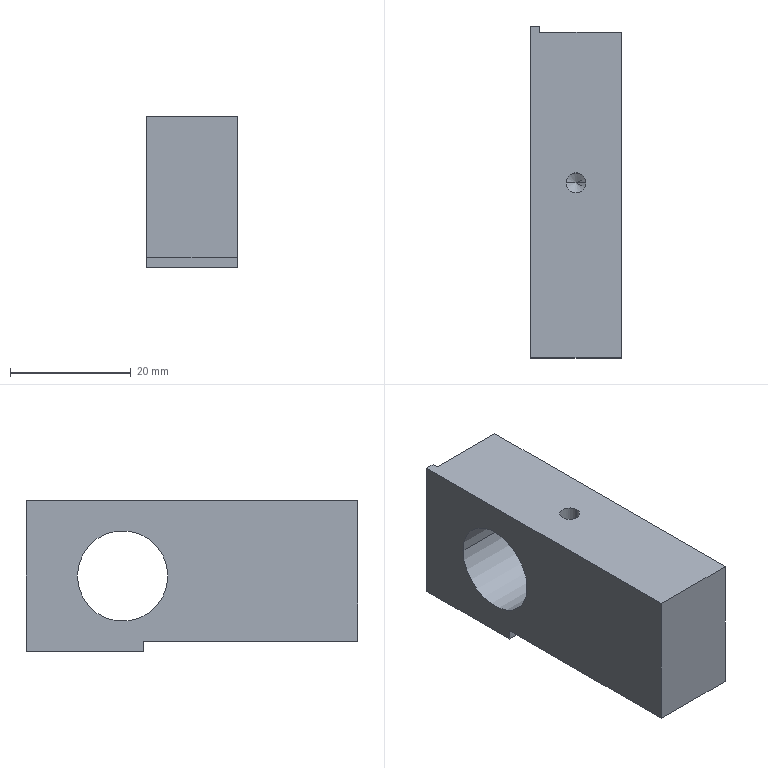Part | STEP file | 11-FG-B07911 | 1 solid | 40 faces | box 15 x 55 x 25 mm | volume 16309 mm3 | cylinder 16 | cone 14 | plane 10 | commonest cylinder face diameters 2.5 x8 3.3 x6 15 x2
STEP:
#1=CARTESIAN_POINT('',(4.7,0.35,9.2));
#2=VERTEX_POINT('',#1);
#3=CARTESIAN_POINT('',(4.7,2.85,9.2));
#4=VERTEX_POINT('',#3);
#5=CARTESIAN_POINT('',(4.7,1.6,9.2));
#6=DIRECTION('',(0.,0.,-1.));
#7=DIRECTION('',(0.,1.,0.));
#8=AXIS2_PLACEMENT_3D('',#5,#6,#7);
#9=CIRCLE('',#8,1.25);
#10=EDGE_CURVE('',#2,#4,#9,.T.);
#11=ORIENTED_EDGE('',*,*,#10,.F.);
#12=CARTESIAN_POINT('',(4.7,0.35,1.7));
#13=VERTEX_POINT('',#12);
#14=CARTESIAN_POINT('',(4.7,0.35,1.7));
#15=DIRECTION('',(0.,0.,-1.));
#16=VECTOR('',#15,1000.);
#17=LINE('',#14,#16);
#18=EDGE_CURVE('',#2,#13,#17,.T.);
#19=ORIENTED_EDGE('',*,*,#18,.T.);
#20=CARTESIAN_POINT('',(4.7,2.85,1.7));
#21=VERTEX_POINT('',#20);
#22=CARTESIAN_POINT('',(4.7,1.6,1.7));
#23=DIRECTION('',(0.,0.,-1.));
#24=DIRECTION('',(0.,1.,0.));
#25=AXIS2_PLACEMENT_3D('',#22,#23,#24);
#26=CIRCLE('',#25,1.25);
#27=EDGE_CURVE('',#13,#21,#26,.T.);
#28=ORIENTED_EDGE('',*,*,#27,.T.);
#29=CARTESIAN_POINT('',(4.7,2.85,1.7));
#30=DIRECTION('',(0.,0.,-1.));
#31=VECTOR('',#30,1000.);
#32=LINE('',#29,#31);
#33=EDGE_CURVE('',#4,#21,#32,.T.);
#34=ORIENTED_EDGE('',*,*,#33,.F.);
#35=EDGE_LOOP('',(#11,#19,#28,#34));
#36=FACE_OUTER_BOUND('',#35,.T.);
#37=CARTESIAN_POINT('',(4.7,1.6,1.7));
#38=DIRECTION('',(0.,0.,-1.));
#39=DIRECTION('',(0.,1.,0.));
#40=AXIS2_PLACEMENT_3D('',#37,#38,#39);
#41=CYLINDRICAL_SURFACE('',#40,1.25);
#42=ADVANCED_FACE('',(#36),#41,.F.);
#43=CARTESIAN_POINT('',(4.7,1.6,9.951));
#44=VERTEX_POINT('',#43);
#45=CARTESIAN_POINT('',(4.7,2.85,9.2));
#46=DIRECTION('',(0.,0.8572,-0.515));
#47=VECTOR('',#46,1000.);
#48=LINE('',#45,#47);
#49=EDGE_CURVE('',#44,#4,#48,.T.);
#50=ORIENTED_EDGE('',*,*,#49,.F.);
#51=CARTESIAN_POINT('',(4.7,0.35,9.2));
#52=DIRECTION('',(0.,-0.8572,-0.515));
#53=VECTOR('',#52,1000.);
#54=LINE('',#51,#53);
#55=EDGE_CURVE('',#44,#2,#54,.T.);
#56=ORIENTED_EDGE('',*,*,#55,.T.);
#57=ORIENTED_EDGE('',*,*,#10,.T.);
#58=EDGE_LOOP('',(#50,#56,#57));
#59=FACE_OUTER_BOUND('',#58,.T.);
#60=CARTESIAN_POINT('',(4.7,1.6,9.2));
#61=DIRECTION('',(0.,0.,-1.));
#62=DIRECTION('',(0.,1.,0.));
#63=AXIS2_PLACEMENT_3D('',#60,#61,#62);
#64=CONICAL_SURFACE('',#63,1.25,1.03);
#65=ADVANCED_FACE('',(#59),#64,.F.);
#66=CARTESIAN_POINT('',(4.7,-19.65,9.2));
#67=VERTEX_POINT('',#66);
#68=CARTESIAN_POINT('',(4.7,-17.15,9.2));
#69=VERTEX_POINT('',#68);
#70=CARTESIAN_POINT('',(4.7,-18.4,9.2));
#71=DIRECTION('',(0.,0.,-1.));
#72=DIRECTION('',(0.,1.,0.));
#73=AXIS2_PLACEMENT_3D('',#70,#71,#72);
#74=CIRCLE('',#73,1.25);
#75=EDGE_CURVE('',#67,#69,#74,.T.);
#76=ORIENTED_EDGE('',*,*,#75,.F.);
#77=CARTESIAN_POINT('',(4.7,-19.65,1.7));
#78=VERTEX_POINT('',#77);
#79=CARTESIAN_POINT('',(4.7,-19.65,1.7));
#80=DIRECTION('',(0.,0.,-1.));
#81=VECTOR('',#80,1000.);
#82=LINE('',#79,#81);
#83=EDGE_CURVE('',#67,#78,#82,.T.);
#84=ORIENTED_EDGE('',*,*,#83,.T.);
#85=CARTESIAN_POINT('',(4.7,-17.15,1.7));
#86=VERTEX_POINT('',#85);
#87=CARTESIAN_POINT('',(4.7,-18.4,1.7));
#88=DIRECTION('',(0.,0.,-1.));
#89=DIRECTION('',(0.,1.,0.));
#90=AXIS2_PLACEMENT_3D('',#87,#88,#89);
#91=CIRCLE('',#90,1.25);
#92=EDGE_CURVE('',#78,#86,#91,.T.);
#93=ORIENTED_EDGE('',*,*,#92,.T.);
#94=CARTESIAN_POINT('',(4.7,-17.15,1.7));
#95=DIRECTION('',(0.,0.,-1.));
#96=VECTOR('',#95,1000.);
#97=LINE('',#94,#96);
#98=EDGE_CURVE('',#69,#86,#97,.T.);
#99=ORIENTED_EDGE('',*,*,#98,.F.);
#100=EDGE_LOOP('',(#76,#84,#93,#99));
#101=FACE_OUTER_BOUND('',#100,.T.);
#102=CARTESIAN_POINT('',(4.7,-18.4,1.7));
#103=DIRECTION('',(0.,0.,-1.));
#104=DIRECTION('',(0.,1.,0.));
#105=AXIS2_PLACEMENT_3D('',#102,#103,#104);
#106=CYLINDRICAL_SURFACE('',#105,1.25);
#107=ADVANCED_FACE('',(#101),#106,.F.);
#108=CARTESIAN_POINT('',(4.7,-18.4,9.951));
#109=VERTEX_POINT('',#108);
#110=CARTESIAN_POINT('',(4.7,-17.15,9.2));
#111=DIRECTION('',(0.,0.8572,-0.515));
#112=VECTOR('',#111,1000.);
#113=LINE('',#110,#112);
#114=EDGE_CURVE('',#109,#69,#113,.T.);
#115=ORIENTED_EDGE('',*,*,#114,.F.);
#116=CARTESIAN_POINT('',(4.7,-19.65,9.2));
#117=DIRECTION('',(0.,-0.8572,-0.515));
#118=VECTOR('',#117,1000.);
#119=LINE('',#116,#118);
#120=EDGE_CURVE('',#109,#67,#119,.T.);
#121=ORIENTED_EDGE('',*,*,#120,.T.);
#122=ORIENTED_EDGE('',*,*,#75,.T.);
#123=EDGE_LOOP('',(#115,#121,#122));
#124=FACE_OUTER_BOUND('',#123,.T.);
#125=CARTESIAN_POINT('',(4.7,-18.4,9.2));
#126=DIRECTION('',(0.,0.,-1.));
#127=DIRECTION('',(0.,1.,0.));
#128=AXIS2_PLACEMENT_3D('',#125,#126,#127);
#129=CONICAL_SURFACE('',#128,1.25,1.03);
#130=ADVANCED_FACE('',(#124),#129,.F.);
#131=CARTESIAN_POINT('',(5.85,5.,14.9));
#132=VERTEX_POINT('',#131);
#133=CARTESIAN_POINT('',(9.15,5.,14.9));
#134=VERTEX_POINT('',#133);
#135=CARTESIAN_POINT('',(7.5,5.,14.9));
#136=DIRECTION('',(0.,0.,1.));
#137=DIRECTION('',(1.,0.,0.));
#138=AXIS2_PLACEMENT_3D('',#135,#136,#137);
#139=CIRCLE('',#138,1.65);
#140=EDGE_CURVE('',#132,#134,#139,.T.);
#141=ORIENTED_EDGE('',*,*,#140,.F.);
#142=CARTESIAN_POINT('',(5.85,5.,25.));
#143=VERTEX_POINT('',#142);
#144=CARTESIAN_POINT('',(5.85,5.,25.));
#145=DIRECTION('',(0.,0.,1.));
#146=VECTOR('',#145,1000.);
#147=LINE('',#144,#146);
#148=EDGE_CURVE('',#132,#143,#147,.T.);
#149=ORIENTED_EDGE('',*,*,#148,.T.);
#150=CARTESIAN_POINT('',(9.15,5.,25.));
#151=VERTEX_POINT('',#150);
#152=CARTESIAN_POINT('',(7.5,5.,25.));
#153=DIRECTION('',(0.,0.,1.));
#154=DIRECTION('',(1.,0.,0.));
#155=AXIS2_PLACEMENT_3D('',#152,#153,#154);
#156=CIRCLE('',#155,1.65);
#157=EDGE_CURVE('',#143,#151,#156,.T.);
#158=ORIENTED_EDGE('',*,*,#157,.T.);
#159=CARTESIAN_POINT('',(9.15,5.,25.));
#160=DIRECTION('',(0.,0.,1.));
#161=VECTOR('',#160,1000.);
#162=LINE('',#159,#161);
#163=EDGE_CURVE('',#134,#151,#162,.T.);
#164=ORIENTED_EDGE('',*,*,#163,.F.);
#165=EDGE_LOOP('',(#141,#149,#158,#164));
#166=FACE_OUTER_BOUND('',#165,.T.);
#167=CARTESIAN_POINT('',(7.5,5.,25.));
#168=DIRECTION('',(0.,0.,1.));
#169=DIRECTION('',(1.,0.,0.));
#170=AXIS2_PLACEMENT_3D('',#167,#168,#169);
#171=CYLINDRICAL_SURFACE('',#170,1.65);
#172=ADVANCED_FACE('',(#166),#171,.F.);
#173=CARTESIAN_POINT('',(7.5,5.,13.909));
#174=VERTEX_POINT('',#173);
#175=CARTESIAN_POINT('',(9.15,5.,14.9));
#176=DIRECTION('',(0.8572,0.,0.515));
#177=VECTOR('',#176,1000.);
#178=LINE('',#175,#177);
#179=EDGE_CURVE('',#174,#134,#178,.T.);
#180=ORIENTED_EDGE('',*,*,#179,.F.);
#181=CARTESIAN_POINT('',(5.85,5.,14.9));
#182=DIRECTION('',(-0.8572,0.,0.515));
#183=VECTOR('',#182,1000.);
#184=LINE('',#181,#183);
#185=EDGE_CURVE('',#174,#132,#184,.T.);
#186=ORIENTED_EDGE('',*,*,#185,.T.);
#187=ORIENTED_EDGE('',*,*,#140,.T.);
#188=EDGE_LOOP('',(#180,#186,#187));
#189=FACE_OUTER_BOUND('',#188,.T.);
#190=CARTESIAN_POINT('',(7.5,5.,14.9));
#191=DIRECTION('',(0.,0.,1.));
#192=DIRECTION('',(1.,0.,0.));
#193=AXIS2_PLACEMENT_3D('',#190,#191,#192);
#194=CONICAL_SURFACE('',#193,1.65,1.03);
#195=ADVANCED_FACE('',(#189),#194,.F.);
#196=CARTESIAN_POINT('',(7.5,-18.5,15.25));
#197=VERTEX_POINT('',#196);
#198=CARTESIAN_POINT('',(7.5,-18.5,12.75));
#199=VERTEX_POINT('',#198);
#200=CARTESIAN_POINT('',(7.5,-18.5,14.));
#201=DIRECTION('',(1.,0.,0.));
#202=DIRECTION('',(0.,0.,-1.));
#203=AXIS2_PLACEMENT_3D('',#200,#201,#202);
#204=CIRCLE('',#203,1.25);
#205=EDGE_CURVE('',#197,#199,#204,.T.);
#206=ORIENTED_EDGE('',*,*,#205,.F.);
#207=CARTESIAN_POINT('',(15.,-18.5,15.25));
#208=VERTEX_POINT('',#207);
#209=CARTESIAN_POINT('',(15.,-18.5,15.25));
#210=DIRECTION('',(1.,0.,0.));
#211=VECTOR('',#210,1000.);
#212=LINE('',#209,#211);
#213=EDGE_CURVE('',#197,#208,#212,.T.);
#214=ORIENTED_EDGE('',*,*,#213,.T.);
#215=CARTESIAN_POINT('',(15.,-18.5,12.75));
#216=VERTEX_POINT('',#215);
#217=CARTESIAN_POINT('',(15.,-18.5,14.));
#218=DIRECTION('',(1.,0.,0.));
#219=DIRECTION('',(0.,0.,-1.));
#220=AXIS2_PLACEMENT_3D('',#217,#218,#219);
#221=CIRCLE('',#220,1.25);
#222=EDGE_CURVE('',#208,#216,#221,.T.);
#223=ORIENTED_EDGE('',*,*,#222,.T.);
#224=CARTESIAN_POINT('',(15.,-18.5,12.75));
#225=DIRECTION('',(1.,0.,0.));
#226=VECTOR('',#225,1000.);
#227=LINE('',#224,#226);
#228=EDGE_CURVE('',#199,#216,#227,.T.);
#229=ORIENTED_EDGE('',*,*,#228,.F.);
#230=EDGE_LOOP('',(#206,#214,#223,#229));
#231=FACE_OUTER_BOUND('',#230,.T.);
#232=CARTESIAN_POINT('',(15.,-18.5,14.));
#233=DIRECTION('',(1.,0.,0.));
#234=DIRECTION('',(0.,0.,-1.));
#235=AXIS2_PLACEMENT_3D('',#232,#233,#234);
#236=CYLINDRICAL_SURFACE('',#235,1.25);
#237=ADVANCED_FACE('',(#231),#236,.F.);
#238=CARTESIAN_POINT('',(6.749,-18.5,14.));
#239=VERTEX_POINT('',#238);
#240=CARTESIAN_POINT('',(7.5,-18.5,12.75));
#241=DIRECTION('',(0.515,0.,-0.8572));
#242=VECTOR('',#241,1000.);
#243=LINE('',#240,#242);
#244=EDGE_CURVE('',#239,#199,#243,.T.);
#245=ORIENTED_EDGE('',*,*,#244,.F.);
#246=CARTESIAN_POINT('',(7.5,-18.5,15.25));
#247=DIRECTION('',(0.515,0.,0.8572));
#248=VECTOR('',#247,1000.);
#249=LINE('',#246,#248);
#250=EDGE_CURVE('',#239,#197,#249,.T.);
#251=ORIENTED_EDGE('',*,*,#250,.T.);
#252=ORIENTED_EDGE('',*,*,#205,.T.);
#253=EDGE_LOOP('',(#245,#251,#252));
#254=FACE_OUTER_BOUND('',#253,.T.);
#255=CARTESIAN_POINT('',(7.5,-18.5,14.));
#256=DIRECTION('',(1.,0.,0.));
#257=DIRECTION('',(0.,0.,-1.));
#258=AXIS2_PLACEMENT_3D('',#255,#256,#257);
#259=CONICAL_SURFACE('',#258,1.25,1.03);
#260=ADVANCED_FACE('',(#254),#259,.F.);
#261=CARTESIAN_POINT('',(7.5,-18.5,7.25));
#262=VERTEX_POINT('',#261);
#263=CARTESIAN_POINT('',(7.5,-18.5,4.75));
#264=VERTEX_POINT('',#263);
#265=CARTESIAN_POINT('',(7.5,-18.5,6.));
#266=DIRECTION('',(1.,0.,0.));
#267=DIRECTION('',(0.,0.,-1.));
#268=AXIS2_PLACEMENT_3D('',#265,#266,#267);
#269=CIRCLE('',#268,1.25);
#270=EDGE_CURVE('',#262,#264,#269,.T.);
#271=ORIENTED_EDGE('',*,*,#270,.F.);
#272=CARTESIAN_POINT('',(15.,-18.5,7.25));
#273=VERTEX_POINT('',#272);
#274=CARTESIAN_POINT('',(15.,-18.5,7.25));
#275=DIRECTION('',(1.,0.,0.));
#276=VECTOR('',#275,1000.);
#277=LINE('',#274,#276);
#278=EDGE_CURVE('',#262,#273,#277,.T.);
#279=ORIENTED_EDGE('',*,*,#278,.T.);
#280=CARTESIAN_POINT('',(15.,-18.5,4.75));
#281=VERTEX_POINT('',#280);
#282=CARTESIAN_POINT('',(15.,-18.5,6.));
#283=DIRECTION('',(1.,0.,0.));
#284=DIRECTION('',(0.,0.,-1.));
#285=AXIS2_PLACEMENT_3D('',#282,#283,#284);
#286=CIRCLE('',#285,1.25);
#287=EDGE_CURVE('',#273,#281,#286,.T.);
#288=ORIENTED_EDGE('',*,*,#287,.T.);
#289=CARTESIAN_POINT('',(15.,-18.5,4.75));
#290=DIRECTION('',(1.,0.,0.));
#291=VECTOR('',#290,1000.);
#292=LINE('',#289,#291);
#293=EDGE_CURVE('',#264,#281,#292,.T.);
#294=ORIENTED_EDGE('',*,*,#293,.F.);
#295=EDGE_LOOP('',(#271,#279,#288,#294));
#296=FACE_OUTER_BOUND('',#295,.T.);
#297=CARTESIAN_POINT('',(15.,-18.5,6.));
#298=DIRECTION('',(1.,0.,0.));
#299=DIRECTION('',(0.,0.,-1.));
#300=AXIS2_PLACEMENT_3D('',#297,#298,#299);
#301=CYLINDRICAL_SURFACE('',#300,1.25);
#302=ADVANCED_FACE('',(#296),#301,.F.);
#303=CARTESIAN_POINT('',(6.749,-18.5,6.));
#304=VERTEX_POINT('',#303);
#305=CARTESIAN_POINT('',(7.5,-18.5,4.75));
#306=DIRECTION('',(0.515,0.,-0.8572));
#307=VECTOR('',#306,1000.);
#308=LINE('',#305,#307);
#309=EDGE_CURVE('',#304,#264,#308,.T.);
#310=ORIENTED_EDGE('',*,*,#309,.F.);
#311=CARTESIAN_POINT('',(7.5,-18.5,7.25));
#312=DIRECTION('',(0.515,0.,0.8572));
#313=VECTOR('',#312,1000.);
#314=LINE('',#311,#313);
#315=EDGE_CURVE('',#304,#262,#314,.T.);
#316=ORIENTED_EDGE('',*,*,#315,.T.);
#317=ORIENTED_EDGE('',*,*,#270,.T.);
#318=EDGE_LOOP('',(#310,#316,#317));
#319=FACE_OUTER_BOUND('',#318,.T.);
#320=CARTESIAN_POINT('',(7.5,-18.5,6.));
#321=DIRECTION('',(1.,0.,0.));
#322=DIRECTION('',(0.,0.,-1.));
#323=AXIS2_PLACEMENT_3D('',#320,#321,#322);
#324=CONICAL_SURFACE('',#323,1.25,1.03);
#325=ADVANCED_FACE('',(#319),#324,.F.);
#326=CARTESIAN_POINT('',(6.5,19.9,3.35));
#327=VERTEX_POINT('',#326);
#328=CARTESIAN_POINT('',(6.5,19.9,6.65));
#329=VERTEX_POINT('',#328);
#330=CARTESIAN_POINT('',(6.5,19.9,5.));
#331=DIRECTION('',(0.,1.,0.));
#332=DIRECTION('',(0.,0.,1.));
#333=AXIS2_PLACEMENT_3D('',#330,#331,#332);
#334=CIRCLE('',#333,1.65);
#335=EDGE_CURVE('',#327,#329,#334,.T.);
#336=ORIENTED_EDGE('',*,*,#335,.F.);
#337=CARTESIAN_POINT('',(6.5,30.,3.35));
#338=VERTEX_POINT('',#337);
#339=CARTESIAN_POINT('',(6.5,30.,3.35));
#340=DIRECTION('',(0.,1.,0.));
#341=VECTOR('',#340,1000.);
#342=LINE('',#339,#341);
#343=EDGE_CURVE('',#327,#338,#342,.T.);
#344=ORIENTED_EDGE('',*,*,#343,.T.);
#345=CARTESIAN_POINT('',(6.5,30.,6.65));
#346=VERTEX_POINT('',#345);
#347=CARTESIAN_POINT('',(6.5,30.,5.));
#348=DIRECTION('',(0.,1.,0.));
#349=DIRECTION('',(0.,0.,1.));
#350=AXIS2_PLACEMENT_3D('',#347,#348,#349);
#351=CIRCLE('',#350,1.65);
#352=EDGE_CURVE('',#338,#346,#351,.T.);
#353=ORIENTED_EDGE('',*,*,#352,.T.);
#354=CARTESIAN_POINT('',(6.5,30.,6.65));
#355=DIRECTION('',(0.,1.,0.));
#356=VECTOR('',#355,1000.);
#357=LINE('',#354,#356);
#358=EDGE_CURVE('',#329,#346,#357,.T.);
#359=ORIENTED_EDGE('',*,*,#358,.F.);
#360=EDGE_LOOP('',(#336,#344,#353,#359));
#361=FACE_OUTER_BOUND('',#360,.T.);
#362=CARTESIAN_POINT('',(6.5,30.,5.));
#363=DIRECTION('',(0.,1.,0.));
#364=DIRECTION('',(0.,0.,1.));
#365=AXIS2_PLACEMENT_3D('',#362,#363,#364);
#366=CYLINDRICAL_SURFACE('',#365,1.65);
#367=ADVANCED_FACE('',(#361),#366,.F.);
#368=CARTESIAN_POINT('',(6.5,18.909,5.));
#369=VERTEX_POINT('',#368);
#370=CARTESIAN_POINT('',(6.5,19.9,6.65));
#371=DIRECTION('',(0.,0.515,0.8572));
#372=VECTOR('',#371,1000.);
#373=LINE('',#370,#372);
#374=EDGE_CURVE('',#369,#329,#373,.T.);
#375=ORIENTED_EDGE('',*,*,#374,.F.);
#376=CARTESIAN_POINT('',(6.5,19.9,3.35));
#377=DIRECTION('',(0.,0.515,-0.8572));
#378=VECTOR('',#377,1000.);
#379=LINE('',#376,#378);
#380=EDGE_CURVE('',#369,#327,#379,.T.);
#381=ORIENTED_EDGE('',*,*,#380,.T.);
#382=ORIENTED_EDGE('',*,*,#335,.T.);
#383=EDGE_LOOP('',(#375,#381,#382));
#384=FACE_OUTER_BOUND('',#383,.T.);
#385=CARTESIAN_POINT('',(6.5,19.9,5.));
#386=DIRECTION('',(0.,1.,0.));
#387=DIRECTION('',(0.,0.,1.));
#388=AXIS2_PLACEMENT_3D('',#385,#386,#387);
#389=CONICAL_SURFACE('',#388,1.65,1.03);
#390=ADVANCED_FACE('',(#384),#389,.F.);
#391=CARTESIAN_POINT('',(6.5,19.9,18.35));
#392=VERTEX_POINT('',#391);
#393=CARTESIAN_POINT('',(6.5,19.9,21.65));
#394=VERTEX_POINT('',#393);
#395=CARTESIAN_POINT('',(6.5,19.9,20.));
#396=DIRECTION('',(0.,1.,0.));
#397=DIRECTION('',(0.,0.,1.));
#398=AXIS2_PLACEMENT_3D('',#395,#396,#397);
#399=CIRCLE('',#398,1.65);
#400=EDGE_CURVE('',#392,#394,#399,.T.);
#401=ORIENTED_EDGE('',*,*,#400,.F.);
#402=CARTESIAN_POINT('',(6.5,30.,18.35));
#403=VERTEX_POINT('',#402);
#404=CARTESIAN_POINT('',(6.5,30.,18.35));
#405=DIRECTION('',(0.,1.,0.));
#406=VECTOR('',#405,1000.);
#407=LINE('',#404,#406);
#408=EDGE_CURVE('',#392,#403,#407,.T.);
#409=ORIENTED_EDGE('',*,*,#408,.T.);
#410=CARTESIAN_POINT('',(6.5,30.,21.65));
#411=VERTEX_POINT('',#410);
#412=CARTESIAN_POINT('',(6.5,30.,20.));
#413=DIRECTION('',(0.,1.,0.));
#414=DIRECTION('',(0.,0.,1.));
#415=AXIS2_PLACEMENT_3D('',#412,#413,#414);
#416=CIRCLE('',#415,1.65);
#417=EDGE_CURVE('',#403,#411,#416,.T.);
#418=ORIENTED_EDGE('',*,*,#417,.T.);
#419=CARTESIAN_POINT('',(6.5,30.,21.65));
#420=DIRECTION('',(0.,1.,0.));
#421=VECTOR('',#420,1000.);
#422=LINE('',#419,#421);
#423=EDGE_CURVE('',#394,#411,#422,.T.);
#424=ORIENTED_EDGE('',*,*,#423,.F.);
#425=EDGE_LOOP('',(#401,#409,#418,#424));
#426=FACE_OUTER_BOUND('',#425,.T.);
#427=CARTESIAN_POINT('',(6.5,30.,20.));
#428=DIRECTION('',(0.,1.,0.));
#429=DIRECTION('',(0.,0.,1.));
#430=AXIS2_PLACEMENT_3D('',#427,#428,#429);
#431=CYLINDRICAL_SURFACE('',#430,1.65);
#432=ADVANCED_FACE('',(#426),#431,.F.);
#433=CARTESIAN_POINT('',(6.5,18.909,20.));
#434=VERTEX_POINT('',#433);
#435=CARTESIAN_POINT('',(6.5,19.9,21.65));
#436=DIRECTION('',(0.,0.515,0.8572));
#437=VECTOR('',#436,1000.);
#438=LINE('',#435,#437);
#439=EDGE_CURVE('',#434,#394,#438,.T.);
#440=ORIENTED_EDGE('',*,*,#439,.F.);
#441=CARTESIAN_POINT('',(6.5,19.9,18.35));
#442=DIRECTION('',(0.,0.515,-0.8572));
#443=VECTOR('',#442,1000.);
#444=LINE('',#441,#443);
#445=EDGE_CURVE('',#434,#392,#444,.T.);
#446=ORIENTED_EDGE('',*,*,#445,.T.);
#447=ORIENTED_EDGE('',*,*,#400,.T.);
#448=EDGE_LOOP('',(#440,#446,#447));
#449=FACE_OUTER_BOUND('',#448,.T.);
#450=CARTESIAN_POINT('',(6.5,19.9,20.));
#451=DIRECTION('',(0.,1.,0.));
#452=DIRECTION('',(0.,0.,1.));
#453=AXIS2_PLACEMENT_3D('',#450,#451,#452);
#454=CONICAL_SURFACE('',#453,1.65,1.03);
#455=ADVANCED_FACE('',(#449),#454,.F.);
#456=CARTESIAN_POINT('',(15.,22.5,12.5));
#457=VERTEX_POINT('',#456);
#458=CARTESIAN_POINT('',(15.,7.5,12.5));
#459=VERTEX_POINT('',#458);
#460=CARTESIAN_POINT('',(15.,15.,12.5));
#461=DIRECTION('',(-1.,0.,0.));
#462=DIRECTION('',(0.,-1.,0.));
#463=AXIS2_PLACEMENT_3D('',#460,#461,#462);
#464=CIRCLE('',#463,7.5);
#465=EDGE_CURVE('',#457,#459,#464,.T.);
#466=ORIENTED_EDGE('',*,*,#465,.F.);
#467=CARTESIAN_POINT('',(0.,22.5,12.5));
#468=VERTEX_POINT('',#467);
#469=CARTESIAN_POINT('',(15.,22.5,12.5));
#470=DIRECTION('',(-1.,0.,0.));
#471=VECTOR('',#470,1000.);
#472=LINE('',#469,#471);
#473=EDGE_CURVE('',#457,#468,#472,.T.);
#474=ORIENTED_EDGE('',*,*,#473,.T.);
#475=CARTESIAN_POINT('',(0.,7.5,12.5));
#476=VERTEX_POINT('',#475);
#477=CARTESIAN_POINT('',(0.,15.,12.5));
#478=DIRECTION('',(-1.,0.,0.));
#479=DIRECTION('',(0.,-1.,0.));
#480=AXIS2_PLACEMENT_3D('',#477,#478,#479);
#481=CIRCLE('',#480,7.5);
#482=EDGE_CURVE('',#468,#476,#481,.T.);
#483=ORIENTED_EDGE('',*,*,#482,.T.);
#484=CARTESIAN_POINT('',(15.,7.5,12.5));
#485=DIRECTION('',(-1.,0.,0.));
#486=VECTOR('',#485,1000.);
#487=LINE('',#484,#486);
#488=EDGE_CURVE('',#459,#476,#487,.T.);
#489=ORIENTED_EDGE('',*,*,#488,.F.);
#490=EDGE_LOOP('',(#466,#474,#483,#489));
#491=FACE_OUTER_BOUND('',#490,.T.);
#492=CARTESIAN_POINT('',(15.,15.,12.5));
#493=DIRECTION('',(-1.,0.,0.));
#494=DIRECTION('',(0.,-1.,0.));
#495=AXIS2_PLACEMENT_3D('',#492,#493,#494);
#496=CYLINDRICAL_SURFACE('',#495,7.5);
#497=ADVANCED_FACE('',(#491),#496,.F.);
#498=CARTESIAN_POINT('',(6.5,30.,20.));
#499=DIRECTION('',(0.,1.,0.));
#500=DIRECTION('',(0.,0.,1.));
#501=AXIS2_PLACEMENT_3D('',#498,#499,#500);
#502=CIRCLE('',#501,1.65);
#503=EDGE_CURVE('',#411,#403,#502,.T.);
#504=ORIENTED_EDGE('',*,*,#503,.F.);
#505=ORIENTED_EDGE('',*,*,#417,.F.);
#506=EDGE_LOOP('',(#504,#505));
#507=FACE_BOUND('',#506,.T.);
#508=CARTESIAN_POINT('',(6.5,30.,5.));
#509=DIRECTION('',(0.,1.,0.));
#510=DIRECTION('',(0.,0.,1.));
#511=AXIS2_PLACEMENT_3D('',#508,#509,#510);
#512=CIRCLE('',#511,1.65);
#513=EDGE_CURVE('',#346,#338,#512,.T.);
#514=ORIENTED_EDGE('',*,*,#513,.F.);
#515=ORIENTED_EDGE('',*,*,#352,.F.);
#516=EDGE_LOOP('',(#514,#515));
#517=FACE_BOUND('',#516,.T.);
#518=CARTESIAN_POINT('',(1.5,30.,25.));
#519=VERTEX_POINT('',#518);
#520=CARTESIAN_POINT('',(1.5,30.,0.));
#521=VERTEX_POINT('',#520);
#522=CARTESIAN_POINT('',(1.5,30.,0.));
#523=DIRECTION('',(0.,0.,-1.));
#524=VECTOR('',#523,1000.);
#525=LINE('',#522,#524);
#526=EDGE_CURVE('',#519,#521,#525,.T.);
#527=ORIENTED_EDGE('',*,*,#526,.F.);
#528=CARTESIAN_POINT('',(15.,30.,25.));
#529=VERTEX_POINT('',#528);
#530=CARTESIAN_POINT('',(0.,30.,25.));
#531=DIRECTION('',(-1.,0.,0.));
#532=VECTOR('',#531,1000.);
#533=LINE('',#530,#532);
#534=EDGE_CURVE('',#529,#519,#533,.T.);
#535=ORIENTED_EDGE('',*,*,#534,.F.);
#536=CARTESIAN_POINT('',(15.,30.,0.));
#537=VERTEX_POINT('',#536);
#538=CARTESIAN_POINT('',(15.,30.,25.));
#539=DIRECTION('',(0.,0.,-1.));
#540=VECTOR('',#539,1000.);
#541=LINE('',#538,#540);
#542=EDGE_CURVE('',#529,#537,#541,.T.);
#543=ORIENTED_EDGE('',*,*,#542,.T.);
#544=CARTESIAN_POINT('',(0.,30.,0.));
#545=DIRECTION('',(-1.,0.,0.));
#546=VECTOR('',#545,1000.);
#547=LINE('',#544,#546);
#548=EDGE_CURVE('',#537,#521,#547,.T.);
#549=ORIENTED_EDGE('',*,*,#548,.T.);
#550=EDGE_LOOP('',(#527,#535,#543,#549));
#551=FACE_OUTER_BOUND('',#550,.T.);
#552=CARTESIAN_POINT('',(0.,30.,25.));
#553=DIRECTION('',(0.,-1.,0.));
#554=DIRECTION('',(0.,0.,-1.));
#555=AXIS2_PLACEMENT_3D('',#552,#553,#554);
#556=PLANE('',#555);
#557=ADVANCED_FACE('',(#507,#517,#551),#556,.F.);
#558=CARTESIAN_POINT('',(0.,15.,12.5));
#559=DIRECTION('',(-1.,0.,0.));
#560=DIRECTION('',(0.,-1.,0.));
#561=AXIS2_PLACEMENT_3D('',#558,#559,#560);
#562=CIRCLE('',#561,7.5);
#563=EDGE_CURVE('',#476,#468,#562,.T.);
#564=ORIENTED_EDGE('',*,*,#563,.F.);
#565=ORIENTED_EDGE('',*,*,#482,.F.);
#566=EDGE_LOOP('',(#564,#565));
#567=FACE_BOUND('',#566,.T.);
#568=CARTESIAN_POINT('',(0.,11.6,0.));
#569=VERTEX_POINT('',#568);
#570=CARTESIAN_POINT('',(0.,11.6,1.7));
#571=VERTEX_POINT('',#570);
#572=CARTESIAN_POINT('',(0.,11.6,25.));
#573=DIRECTION('',(0.,0.,1.));
#574=VECTOR('',#573,1000.);
#575=LINE('',#572,#574);
#576=EDGE_CURVE('',#569,#571,#575,.T.);
#577=ORIENTED_EDGE('',*,*,#576,.T.);
#578=CARTESIAN_POINT('',(0.,-24.,1.7));
#579=VERTEX_POINT('',#578);
#580=CARTESIAN_POINT('',(0.,0.,1.7));
#581=DIRECTION('',(0.,-1.,0.));
#582=VECTOR('',#581,1000.);
#583=LINE('',#580,#582);
#584=EDGE_CURVE('',#571,#579,#583,.T.);
#585=ORIENTED_EDGE('',*,*,#584,.T.);
#586=CARTESIAN_POINT('',(0.,-24.,25.));
#587=VERTEX_POINT('',#586);
#588=CARTESIAN_POINT('',(0.,-24.,25.));
#589=DIRECTION('',(0.,0.,-1.));
#590=VECTOR('',#589,1000.);
#591=LINE('',#588,#590);
#592=EDGE_CURVE('',#587,#579,#591,.T.);
#593=ORIENTED_EDGE('',*,*,#592,.F.);
#594=CARTESIAN_POINT('',(0.,31.,25.));
#595=VERTEX_POINT('',#594);
#596=CARTESIAN_POINT('',(0.,0.,25.));
#597=DIRECTION('',(0.,-1.,0.));
#598=VECTOR('',#597,1000.);
#599=LINE('',#596,#598);
#600=EDGE_CURVE('',#595,#587,#599,.T.);
#601=ORIENTED_EDGE('',*,*,#600,.F.);
#602=CARTESIAN_POINT('',(0.,31.,0.));
#603=VERTEX_POINT('',#602);
#604=CARTESIAN_POINT('',(0.,31.,0.));
#605=DIRECTION('',(0.,0.,1.));
#606=VECTOR('',#605,1000.);
#607=LINE('',#604,#606);
#608=EDGE_CURVE('',#603,#595,#607,.T.);
#609=ORIENTED_EDGE('',*,*,#608,.F.);
#610=CARTESIAN_POINT('',(0.,0.,0.));
#611=DIRECTION('',(0.,-1.,0.));
#612=VECTOR('',#611,1000.);
#613=LINE('',#610,#612);
#614=EDGE_CURVE('',#603,#569,#613,.T.);
#615=ORIENTED_EDGE('',*,*,#614,.T.);
#616=EDGE_LOOP('',(#577,#585,#593,#601,#609,#615));
#617=FACE_OUTER_BOUND('',#616,.T.);
#618=CARTESIAN_POINT('',(0.,0.,25.));
#619=DIRECTION('',(1.,0.,0.));
#620=DIRECTION('',(0.,1.,0.));
#621=AXIS2_PLACEMENT_3D('',#618,#619,#620);
#622=PLANE('',#621);
#623=ADVANCED_FACE('',(#567,#617),#622,.F.);
#624=CARTESIAN_POINT('',(15.,-18.5,14.));
#625=DIRECTION('',(1.,0.,0.));
#626=DIRECTION('',(0.,0.,-1.));
#627=AXIS2_PLACEMENT_3D('',#624,#625,#626);
#628=CIRCLE('',#627,1.25);
#629=EDGE_CURVE('',#216,#208,#628,.T.);
#630=ORIENTED_EDGE('',*,*,#629,.F.);
#631=ORIENTED_EDGE('',*,*,#222,.F.);
#632=EDGE_LOOP('',(#630,#631));
#633=FACE_BOUND('',#632,.T.);
#634=CARTESIAN_POINT('',(15.,-18.5,6.));
#635=DIRECTION('',(1.,0.,0.));
#636=DIRECTION('',(0.,0.,-1.));
#637=AXIS2_PLACEMENT_3D('',#634,#635,#636);
#638=CIRCLE('',#637,1.25);
#639=EDGE_CURVE('',#281,#273,#638,.T.);
#640=ORIENTED_EDGE('',*,*,#639,.F.);
#641=ORIENTED_EDGE('',*,*,#287,.F.);
#642=EDGE_LOOP('',(#640,#641));
#643=FACE_BOUND('',#642,.T.);
#644=CARTESIAN_POINT('',(15.,15.,12.5));
#645=DIRECTION('',(-1.,0.,0.));
#646=DIRECTION('',(0.,-1.,0.));
#647=AXIS2_PLACEMENT_3D('',#644,#645,#646);
#648=CIRCLE('',#647,7.5);
#649=EDGE_CURVE('',#459,#457,#648,.T.);
#650=ORIENTED_EDGE('',*,*,#649,.T.);
#651=ORIENTED_EDGE('',*,*,#465,.T.);
#652=EDGE_LOOP('',(#650,#651));
#653=FACE_BOUND('',#652,.T.);
#654=CARTESIAN_POINT('',(15.,-24.,1.7));
#655=VERTEX_POINT('',#654);
#656=CARTESIAN_POINT('',(15.,-24.,25.));
#657=VERTEX_POINT('',#656);
#658=CARTESIAN_POINT('',(15.,-24.,25.));
#659=DIRECTION('',(0.,0.,1.));
#660=VECTOR('',#659,1000.);
#661=LINE('',#658,#660);
#662=EDGE_CURVE('',#655,#657,#661,.T.);
#663=ORIENTED_EDGE('',*,*,#662,.F.);
#664=CARTESIAN_POINT('',(15.,11.6,1.7));
#665=VERTEX_POINT('',#664);
#666=CARTESIAN_POINT('',(15.,11.6,1.7));
#667=DIRECTION('',(0.,-1.,0.));
#668=VECTOR('',#667,1000.);
#669=LINE('',#666,#668);
#670=EDGE_CURVE('',#665,#655,#669,.T.);
#671=ORIENTED_EDGE('',*,*,#670,.F.);
#672=CARTESIAN_POINT('',(15.,11.6,0.));
#673=VERTEX_POINT('',#672);
#674=CARTESIAN_POINT('',(15.,11.6,0.));
#675=DIRECTION('',(0.,0.,1.));
#676=VECTOR('',#675,1000.);
#677=LINE('',#674,#676);
#678=EDGE_CURVE('',#673,#665,#677,.T.);
#679=ORIENTED_EDGE('',*,*,#678,.F.);
#680=CARTESIAN_POINT('',(15.,0.,0.));
#681=DIRECTION('',(0.,1.,0.));
#682=VECTOR('',#681,1000.);
#683=LINE('',#680,#682);
#684=EDGE_CURVE('',#673,#537,#683,.T.);
#685=ORIENTED_EDGE('',*,*,#684,.T.);
#686=ORIENTED_EDGE('',*,*,#542,.F.);
#687=CARTESIAN_POINT('',(15.,0.,25.));
#688=DIRECTION('',(0.,1.,0.));
#689=VECTOR('',#688,1000.);
#690=LINE('',#687,#689);
#691=EDGE_CURVE('',#657,#529,#690,.T.);
#692=ORIENTED_EDGE('',*,*,#691,.F.);
#693=EDGE_LOOP('',(#663,#671,#679,#685,#686,#692));
#694=FACE_OUTER_BOUND('',#693,.T.);
#695=CARTESIAN_POINT('',(15.,0.,25.));
#696=DIRECTION('',(-1.,0.,0.));
#697=DIRECTION('',(0.,-1.,0.));
#698=AXIS2_PLACEMENT_3D('',#695,#696,#697);
#699=PLANE('',#698);
#700=ADVANCED_FACE('',(#633,#643,#653,#694),#699,.F.);
#701=CARTESIAN_POINT('',(7.5,5.,25.));
#702=DIRECTION('',(0.,0.,1.));
#703=DIRECTION('',(1.,0.,0.));
#704=AXIS2_PLACEMENT_3D('',#701,#702,#703);
#705=CIRCLE('',#704,1.65);
#706=EDGE_CURVE('',#151,#143,#705,.T.);
#707=ORIENTED_EDGE('',*,*,#706,.F.);
#708=ORIENTED_EDGE('',*,*,#157,.F.);
#709=EDGE_LOOP('',(#707,#708));
#710=FACE_BOUND('',#709,.T.);
#711=ORIENTED_EDGE('',*,*,#600,.T.);
#712=CARTESIAN_POINT('',(0.,-24.,25.));
#713=DIRECTION('',(-1.,0.,0.));
#714=VECTOR('',#713,1000.);
#715=LINE('',#712,#714);
#716=EDGE_CURVE('',#657,#587,#715,.T.);
#717=ORIENTED_EDGE('',*,*,#716,.F.);
#718=ORIENTED_EDGE('',*,*,#691,.T.);
#719=ORIENTED_EDGE('',*,*,#534,.T.);
#720=CARTESIAN_POINT('',(1.5,31.,25.));
#721=VERTEX_POINT('',#720);
#722=CARTESIAN_POINT('',(1.5,31.,25.));
#723=DIRECTION('',(0.,-1.,0.));
#724=VECTOR('',#723,1000.);
#725=LINE('',#722,#724);
#726=EDGE_CURVE('',#721,#519,#725,.T.);
#727=ORIENTED_EDGE('',*,*,#726,.F.);
#728=CARTESIAN_POINT('',(0.,31.,25.));
#729=DIRECTION('',(1.,0.,0.));
#730=VECTOR('',#729,1000.);
#731=LINE('',#728,#730);
#732=EDGE_CURVE('',#595,#721,#731,.T.);
#733=ORIENTED_EDGE('',*,*,#732,.F.);
#734=EDGE_LOOP('',(#711,#717,#718,#719,#727,#733));
#735=FACE_OUTER_BOUND('',#734,.T.);
#736=CARTESIAN_POINT('',(0.,30.,25.));
#737=DIRECTION('',(0.,0.,-1.));
#738=DIRECTION('',(-1.,0.,0.));
#739=AXIS2_PLACEMENT_3D('',#736,#737,#738);
#740=PLANE('',#739);
#741=ADVANCED_FACE('',(#710,#735),#740,.F.);
#742=CARTESIAN_POINT('',(-16.,11.6,0.));
#743=DIRECTION('',(1.,0.,0.));
#744=VECTOR('',#743,1000.);
#745=LINE('',#742,#744);
#746=EDGE_CURVE('',#569,#673,#745,.T.);
#747=ORIENTED_EDGE('',*,*,#746,.F.);
#748=ORIENTED_EDGE('',*,*,#614,.F.);
#749=CARTESIAN_POINT('',(1.5,31.,0.));
#750=VERTEX_POINT('',#749);
#751=CARTESIAN_POINT('',(0.,31.,0.));
#752=DIRECTION('',(-1.,0.,0.));
#753=VECTOR('',#752,1000.);
#754=LINE('',#751,#753);
#755=EDGE_CURVE('',#750,#603,#754,.T.);
#756=ORIENTED_EDGE('',*,*,#755,.F.);
#757=CARTESIAN_POINT('',(1.5,31.,0.));
#758=DIRECTION('',(0.,-1.,0.));
#759=VECTOR('',#758,1000.);
#760=LINE('',#757,#759);
#761=EDGE_CURVE('',#750,#521,#760,.T.);
#762=ORIENTED_EDGE('',*,*,#761,.T.);
#763=ORIENTED_EDGE('',*,*,#548,.F.);
#764=ORIENTED_EDGE('',*,*,#684,.F.);
#765=EDGE_LOOP('',(#747,#748,#756,#762,#763,#764));
#766=FACE_OUTER_BOUND('',#765,.T.);
#767=CARTESIAN_POINT('',(0.,30.,0.));
#768=DIRECTION('',(0.,0.,-1.));
#769=DIRECTION('',(-1.,0.,0.));
#770=AXIS2_PLACEMENT_3D('',#767,#768,#769);
#771=PLANE('',#770);
#772=ADVANCED_FACE('',(#766),#771,.T.);
#773=ORIENTED_EDGE('',*,*,#473,.F.);
#774=ORIENTED_EDGE('',*,*,#649,.F.);
#775=ORIENTED_EDGE('',*,*,#488,.T.);
#776=ORIENTED_EDGE('',*,*,#563,.T.);
#777=EDGE_LOOP('',(#773,#774,#775,#776));
#778=FACE_OUTER_BOUND('',#777,.T.);
#779=CARTESIAN_POINT('',(15.,15.,12.5));
#780=DIRECTION('',(-1.,0.,0.));
#781=DIRECTION('',(0.,-1.,0.));
#782=AXIS2_PLACEMENT_3D('',#779,#780,#781);
#783=CYLINDRICAL_SURFACE('',#782,7.5);
#784=ADVANCED_FACE('',(#778),#783,.F.);
#785=ORIENTED_EDGE('',*,*,#445,.F.);
#786=ORIENTED_EDGE('',*,*,#439,.T.);
#787=CARTESIAN_POINT('',(6.5,19.9,20.));
#788=DIRECTION('',(0.,1.,0.));
#789=DIRECTION('',(0.,0.,1.));
#790=AXIS2_PLACEMENT_3D('',#787,#788,#789);
#791=CIRCLE('',#790,1.65);
#792=EDGE_CURVE('',#394,#392,#791,.T.);
#793=ORIENTED_EDGE('',*,*,#792,.T.);
#794=EDGE_LOOP('',(#785,#786,#793));
#795=FACE_OUTER_BOUND('',#794,.T.);
#796=CARTESIAN_POINT('',(6.5,19.9,20.));
#797=DIRECTION('',(0.,1.,0.));
#798=DIRECTION('',(0.,0.,1.));
#799=AXIS2_PLACEMENT_3D('',#796,#797,#798);
#800=CONICAL_SURFACE('',#799,1.65,1.03);
#801=ADVANCED_FACE('',(#795),#800,.F.);
#802=ORIENTED_EDGE('',*,*,#408,.F.);
#803=ORIENTED_EDGE('',*,*,#792,.F.);
#804=ORIENTED_EDGE('',*,*,#423,.T.);
#805=ORIENTED_EDGE('',*,*,#503,.T.);
#806=EDGE_LOOP('',(#802,#803,#804,#805));
#807=FACE_OUTER_BOUND('',#806,.T.);
#808=CARTESIAN_POINT('',(6.5,30.,20.));
#809=DIRECTION('',(0.,1.,0.));
#810=DIRECTION('',(0.,0.,1.));
#811=AXIS2_PLACEMENT_3D('',#808,#809,#810);
#812=CYLINDRICAL_SURFACE('',#811,1.65);
#813=ADVANCED_FACE('',(#807),#812,.F.);
#814=ORIENTED_EDGE('',*,*,#380,.F.);
#815=ORIENTED_EDGE('',*,*,#374,.T.);
#816=CARTESIAN_POINT('',(6.5,19.9,5.));
#817=DIRECTION('',(0.,1.,0.));
#818=DIRECTION('',(0.,0.,1.));
#819=AXIS2_PLACEMENT_3D('',#816,#817,#818);
#820=CIRCLE('',#819,1.65);
#821=EDGE_CURVE('',#329,#327,#820,.T.);
#822=ORIENTED_EDGE('',*,*,#821,.T.);
#823=EDGE_LOOP('',(#814,#815,#822));
#824=FACE_OUTER_BOUND('',#823,.T.);
#825=CARTESIAN_POINT('',(6.5,19.9,5.));
#826=DIRECTION('',(0.,1.,0.));
#827=DIRECTION('',(0.,0.,1.));
#828=AXIS2_PLACEMENT_3D('',#825,#826,#827);
#829=CONICAL_SURFACE('',#828,1.65,1.03);
#830=ADVANCED_FACE('',(#824),#829,.F.);
#831=ORIENTED_EDGE('',*,*,#343,.F.);
#832=ORIENTED_EDGE('',*,*,#821,.F.);
#833=ORIENTED_EDGE('',*,*,#358,.T.);
#834=ORIENTED_EDGE('',*,*,#513,.T.);
#835=EDGE_LOOP('',(#831,#832,#833,#834));
#836=FACE_OUTER_BOUND('',#835,.T.);
#837=CARTESIAN_POINT('',(6.5,30.,5.));
#838=DIRECTION('',(0.,1.,0.));
#839=DIRECTION('',(0.,0.,1.));
#840=AXIS2_PLACEMENT_3D('',#837,#838,#839);
#841=CYLINDRICAL_SURFACE('',#840,1.65);
#842=ADVANCED_FACE('',(#836),#841,.F.);
#843=ORIENTED_EDGE('',*,*,#526,.T.);
#844=ORIENTED_EDGE('',*,*,#761,.F.);
#845=CARTESIAN_POINT('',(1.5,31.,0.));
#846=DIRECTION('',(0.,0.,-1.));
#847=VECTOR('',#846,1000.);
#848=LINE('',#845,#847);
#849=EDGE_CURVE('',#721,#750,#848,.T.);
#850=ORIENTED_EDGE('',*,*,#849,.F.);
#851=ORIENTED_EDGE('',*,*,#726,.T.);
#852=EDGE_LOOP('',(#843,#844,#850,#851));
#853=FACE_OUTER_BOUND('',#852,.T.);
#854=CARTESIAN_POINT('',(1.5,31.,0.));
#855=DIRECTION('',(-1.,0.,0.));
#856=DIRECTION('',(0.,0.,1.));
#857=AXIS2_PLACEMENT_3D('',#854,#855,#856);
#858=PLANE('',#857);
#859=ADVANCED_FACE('',(#853),#858,.F.);
#860=ORIENTED_EDGE('',*,*,#608,.T.);
#861=ORIENTED_EDGE('',*,*,#732,.T.);
#862=ORIENTED_EDGE('',*,*,#849,.T.);
#863=ORIENTED_EDGE('',*,*,#755,.T.);
#864=EDGE_LOOP('',(#860,#861,#862,#863));
#865=FACE_OUTER_BOUND('',#864,.T.);
#866=CARTESIAN_POINT('',(0.,31.,25.));
#867=DIRECTION('',(0.,1.,0.));
#868=DIRECTION('',(0.,0.,1.));
#869=AXIS2_PLACEMENT_3D('',#866,#867,#868);
#870=PLANE('',#869);
#871=ADVANCED_FACE('',(#865),#870,.T.);
#872=CARTESIAN_POINT('',(0.,-24.,1.7));
#873=DIRECTION('',(-1.,0.,0.));
#874=VECTOR('',#873,1000.);
#875=LINE('',#872,#874);
#876=EDGE_CURVE('',#655,#579,#875,.T.);
#877=ORIENTED_EDGE('',*,*,#876,.F.);
#878=ORIENTED_EDGE('',*,*,#662,.T.);
#879=ORIENTED_EDGE('',*,*,#716,.T.);
#880=ORIENTED_EDGE('',*,*,#592,.T.);
#881=EDGE_LOOP('',(#877,#878,#879,#880));
#882=FACE_OUTER_BOUND('',#881,.T.);
#883=CARTESIAN_POINT('',(0.,-24.,0.));
#884=DIRECTION('',(0.,-1.,0.));
#885=DIRECTION('',(0.,0.,-1.));
#886=AXIS2_PLACEMENT_3D('',#883,#884,#885);
#887=PLANE('',#886);
#888=ADVANCED_FACE('',(#882),#887,.T.);
#889=ORIENTED_EDGE('',*,*,#315,.F.);
#890=ORIENTED_EDGE('',*,*,#309,.T.);
#891=CARTESIAN_POINT('',(7.5,-18.5,6.));
#892=DIRECTION('',(1.,0.,0.));
#893=DIRECTION('',(0.,0.,-1.));
#894=AXIS2_PLACEMENT_3D('',#891,#892,#893);
#895=CIRCLE('',#894,1.25);
#896=EDGE_CURVE('',#264,#262,#895,.T.);
#897=ORIENTED_EDGE('',*,*,#896,.T.);
#898=EDGE_LOOP('',(#889,#890,#897));
#899=FACE_OUTER_BOUND('',#898,.T.);
#900=CARTESIAN_POINT('',(7.5,-18.5,6.));
#901=DIRECTION('',(1.,0.,0.));
#902=DIRECTION('',(0.,0.,-1.));
#903=AXIS2_PLACEMENT_3D('',#900,#901,#902);
#904=CONICAL_SURFACE('',#903,1.25,1.03);
#905=ADVANCED_FACE('',(#899),#904,.F.);
#906=ORIENTED_EDGE('',*,*,#278,.F.);
#907=ORIENTED_EDGE('',*,*,#896,.F.);
#908=ORIENTED_EDGE('',*,*,#293,.T.);
#909=ORIENTED_EDGE('',*,*,#639,.T.);
#910=EDGE_LOOP('',(#906,#907,#908,#909));
#911=FACE_OUTER_BOUND('',#910,.T.);
#912=CARTESIAN_POINT('',(15.,-18.5,6.));
#913=DIRECTION('',(1.,0.,0.));
#914=DIRECTION('',(0.,0.,-1.));
#915=AXIS2_PLACEMENT_3D('',#912,#913,#914);
#916=CYLINDRICAL_SURFACE('',#915,1.25);
#917=ADVANCED_FACE('',(#911),#916,.F.);
#918=ORIENTED_EDGE('',*,*,#250,.F.);
#919=ORIENTED_EDGE('',*,*,#244,.T.);
#920=CARTESIAN_POINT('',(7.5,-18.5,14.));
#921=DIRECTION('',(1.,0.,0.));
#922=DIRECTION('',(0.,0.,-1.));
#923=AXIS2_PLACEMENT_3D('',#920,#921,#922);
#924=CIRCLE('',#923,1.25);
#925=EDGE_CURVE('',#199,#197,#924,.T.);
#926=ORIENTED_EDGE('',*,*,#925,.T.);
#927=EDGE_LOOP('',(#918,#919,#926));
#928=FACE_OUTER_BOUND('',#927,.T.);
#929=CARTESIAN_POINT('',(7.5,-18.5,14.));
#930=DIRECTION('',(1.,0.,0.));
#931=DIRECTION('',(0.,0.,-1.));
#932=AXIS2_PLACEMENT_3D('',#929,#930,#931);
#933=CONICAL_SURFACE('',#932,1.25,1.03);
#934=ADVANCED_FACE('',(#928),#933,.F.);
#935=ORIENTED_EDGE('',*,*,#213,.F.);
#936=ORIENTED_EDGE('',*,*,#925,.F.);
#937=ORIENTED_EDGE('',*,*,#228,.T.);
#938=ORIENTED_EDGE('',*,*,#629,.T.);
#939=EDGE_LOOP('',(#935,#936,#937,#938));
#940=FACE_OUTER_BOUND('',#939,.T.);
#941=CARTESIAN_POINT('',(15.,-18.5,14.));
#942=DIRECTION('',(1.,0.,0.));
#943=DIRECTION('',(0.,0.,-1.));
#944=AXIS2_PLACEMENT_3D('',#941,#942,#943);
#945=CYLINDRICAL_SURFACE('',#944,1.25);
#946=ADVANCED_FACE('',(#940),#945,.F.);
#947=ORIENTED_EDGE('',*,*,#746,.T.);
#948=ORIENTED_EDGE('',*,*,#678,.T.);
#949=CARTESIAN_POINT('',(-16.,11.6,1.7));
#950=DIRECTION('',(1.,0.,0.));
#951=VECTOR('',#950,1000.);
#952=LINE('',#949,#951);
#953=EDGE_CURVE('',#571,#665,#952,.T.);
#954=ORIENTED_EDGE('',*,*,#953,.F.);
#955=ORIENTED_EDGE('',*,*,#576,.F.);
#956=EDGE_LOOP('',(#947,#948,#954,#955));
#957=FACE_OUTER_BOUND('',#956,.T.);
#958=CARTESIAN_POINT('',(-16.,11.6,0.));
#959=DIRECTION('',(0.,1.,0.));
#960=DIRECTION('',(-1.,0.,0.));
#961=AXIS2_PLACEMENT_3D('',#958,#959,#960);
#962=PLANE('',#961);
#963=ADVANCED_FACE('',(#957),#962,.F.);
#964=CARTESIAN_POINT('',(4.7,1.6,1.7));
#965=DIRECTION('',(0.,0.,-1.));
#966=DIRECTION('',(0.,1.,0.));
#967=AXIS2_PLACEMENT_3D('',#964,#965,#966);
#968=CIRCLE('',#967,1.25);
#969=EDGE_CURVE('',#21,#13,#968,.T.);
#970=ORIENTED_EDGE('',*,*,#969,.F.);
#971=ORIENTED_EDGE('',*,*,#27,.F.);
#972=EDGE_LOOP('',(#970,#971));
#973=FACE_BOUND('',#972,.T.);
#974=CARTESIAN_POINT('',(4.7,-18.4,1.7));
#975=DIRECTION('',(0.,0.,-1.));
#976=DIRECTION('',(0.,1.,0.));
#977=AXIS2_PLACEMENT_3D('',#974,#975,#976);
#978=CIRCLE('',#977,1.25);
#979=EDGE_CURVE('',#86,#78,#978,.T.);
#980=ORIENTED_EDGE('',*,*,#979,.F.);
#981=ORIENTED_EDGE('',*,*,#92,.F.);
#982=EDGE_LOOP('',(#980,#981));
#983=FACE_BOUND('',#982,.T.);
#984=ORIENTED_EDGE('',*,*,#953,.T.);
#985=ORIENTED_EDGE('',*,*,#670,.T.);
#986=ORIENTED_EDGE('',*,*,#876,.T.);
#987=ORIENTED_EDGE('',*,*,#584,.F.);
#988=EDGE_LOOP('',(#984,#985,#986,#987));
#989=FACE_OUTER_BOUND('',#988,.T.);
#990=CARTESIAN_POINT('',(-16.,11.6,1.7));
#991=DIRECTION('',(0.,0.,1.));
#992=DIRECTION('',(0.,-1.,0.));
#993=AXIS2_PLACEMENT_3D('',#990,#991,#992);
#994=PLANE('',#993);
#995=ADVANCED_FACE('',(#973,#983,#989),#994,.F.);
#996=ORIENTED_EDGE('',*,*,#185,.F.);
#997=ORIENTED_EDGE('',*,*,#179,.T.);
#998=CARTESIAN_POINT('',(7.5,5.,14.9));
#999=DIRECTION('',(0.,0.,1.));
#1000=DIRECTION('',(1.,0.,0.));
#1001=AXIS2_PLACEMENT_3D('',#998,#999,#1000);
#1002=CIRCLE('',#1001,1.65);
#1003=EDGE_CURVE('',#134,#132,#1002,.T.);
#1004=ORIENTED_EDGE('',*,*,#1003,.T.);
#1005=EDGE_LOOP('',(#996,#997,#1004));
#1006=FACE_OUTER_BOUND('',#1005,.T.);
#1007=CARTESIAN_POINT('',(7.5,5.,14.9));
#1008=DIRECTION('',(0.,0.,1.));
#1009=DIRECTION('',(1.,0.,0.));
#1010=AXIS2_PLACEMENT_3D('',#1007,#1008,#1009);
#1011=CONICAL_SURFACE('',#1010,1.65,1.03);
#1012=ADVANCED_FACE('',(#1006),#1011,.F.);
#1013=ORIENTED_EDGE('',*,*,#148,.F.);
#1014=ORIENTED_EDGE('',*,*,#1003,.F.);
#1015=ORIENTED_EDGE('',*,*,#163,.T.);
#1016=ORIENTED_EDGE('',*,*,#706,.T.);
#1017=EDGE_LOOP('',(#1013,#1014,#1015,#1016));
#1018=FACE_OUTER_BOUND('',#1017,.T.);
#1019=CARTESIAN_POINT('',(7.5,5.,25.));
#1020=DIRECTION('',(0.,0.,1.));
#1021=DIRECTION('',(1.,0.,0.));
#1022=AXIS2_PLACEMENT_3D('',#1019,#1020,#1021);
#1023=CYLINDRICAL_SURFACE('',#1022,1.65);
#1024=ADVANCED_FACE('',(#1018),#1023,.F.);
#1025=ORIENTED_EDGE('',*,*,#120,.F.);
#1026=ORIENTED_EDGE('',*,*,#114,.T.);
#1027=CARTESIAN_POINT('',(4.7,-18.4,9.2));
#1028=DIRECTION('',(0.,0.,-1.));
#1029=DIRECTION('',(0.,1.,0.));
#1030=AXIS2_PLACEMENT_3D('',#1027,#1028,#1029);
#1031=CIRCLE('',#1030,1.25);
#1032=EDGE_CURVE('',#69,#67,#1031,.T.);
#1033=ORIENTED_EDGE('',*,*,#1032,.T.);
#1034=EDGE_LOOP('',(#1025,#1026,#1033));
#1035=FACE_OUTER_BOUND('',#1034,.T.);
#1036=CARTESIAN_POINT('',(4.7,-18.4,9.2));
#1037=DIRECTION('',(0.,0.,-1.));
#1038=DIRECTION('',(0.,1.,0.));
#1039=AXIS2_PLACEMENT_3D('',#1036,#1037,#1038);
#1040=CONICAL_SURFACE('',#1039,1.25,1.03);
#1041=ADVANCED_FACE('',(#1035),#1040,.F.);
#1042=ORIENTED_EDGE('',*,*,#83,.F.);
#1043=ORIENTED_EDGE('',*,*,#1032,.F.);
#1044=ORIENTED_EDGE('',*,*,#98,.T.);
#1045=ORIENTED_EDGE('',*,*,#979,.T.);
#1046=EDGE_LOOP('',(#1042,#1043,#1044,#1045));
#1047=FACE_OUTER_BOUND('',#1046,.T.);
#1048=CARTESIAN_POINT('',(4.7,-18.4,1.7));
#1049=DIRECTION('',(0.,0.,-1.));
#1050=DIRECTION('',(0.,1.,0.));
#1051=AXIS2_PLACEMENT_3D('',#1048,#1049,#1050);
#1052=CYLINDRICAL_SURFACE('',#1051,1.25);
#1053=ADVANCED_FACE('',(#1047),#1052,.F.);
#1054=ORIENTED_EDGE('',*,*,#55,.F.);
#1055=ORIENTED_EDGE('',*,*,#49,.T.);
#1056=CARTESIAN_POINT('',(4.7,1.6,9.2));
#1057=DIRECTION('',(0.,0.,-1.));
#1058=DIRECTION('',(0.,1.,0.));
#1059=AXIS2_PLACEMENT_3D('',#1056,#1057,#1058);
#1060=CIRCLE('',#1059,1.25);
#1061=EDGE_CURVE('',#4,#2,#1060,.T.);
#1062=ORIENTED_EDGE('',*,*,#1061,.T.);
#1063=EDGE_LOOP('',(#1054,#1055,#1062));
#1064=FACE_OUTER_BOUND('',#1063,.T.);
#1065=CARTESIAN_POINT('',(4.7,1.6,9.2));
#1066=DIRECTION('',(0.,0.,-1.));
#1067=DIRECTION('',(0.,1.,0.));
#1068=AXIS2_PLACEMENT_3D('',#1065,#1066,#1067);
#1069=CONICAL_SURFACE('',#1068,1.25,1.03);
#1070=ADVANCED_FACE('',(#1064),#1069,.F.);
#1071=ORIENTED_EDGE('',*,*,#18,.F.);
#1072=ORIENTED_EDGE('',*,*,#1061,.F.);
#1073=ORIENTED_EDGE('',*,*,#33,.T.);
#1074=ORIENTED_EDGE('',*,*,#969,.T.);
#1075=EDGE_LOOP('',(#1071,#1072,#1073,#1074));
#1076=FACE_OUTER_BOUND('',#1075,.T.);
#1077=CARTESIAN_POINT('',(4.7,1.6,1.7));
#1078=DIRECTION('',(0.,0.,-1.));
#1079=DIRECTION('',(0.,1.,0.));
#1080=AXIS2_PLACEMENT_3D('',#1077,#1078,#1079);
#1081=CYLINDRICAL_SURFACE('',#1080,1.25);
#1082=ADVANCED_FACE('',(#1076),#1081,.F.);
#1083=CLOSED_SHELL('',(#42,#65,#107,#130,#172,#195,#237,#260,#302,#325,#367,#390,#432,#455,#497,#557,#623,#700,#741,#772,#784,#801,#813,#830,#842,#859,#871,#888,#905,#917,#934,#946,#963,#995,#1012,#1024,#1041,#1053,#1070,#1082));
#1084=MANIFOLD_SOLID_BREP('',#1083);
#1085=CARTESIAN_POINT('',(0.,0.,0.));
#1086=DIRECTION('',(0.,0.,1.));
#1087=DIRECTION('',(1.,0.,0.));
#1088=AXIS2_PLACEMENT_3D('',#1085,#1086,#1087);
#1089=(LENGTH_UNIT()NAMED_UNIT(*)SI_UNIT(.MILLI.,.METRE.));
#1090=UNCERTAINTY_MEASURE_WITH_UNIT(LENGTH_MEASURE(0.00001),#1089,'','');
#1091=(NAMED_UNIT(*)PLANE_ANGLE_UNIT()SI_UNIT($,.RADIAN.));
#1092=(NAMED_UNIT(*)SI_UNIT($,.STERADIAN.)SOLID_ANGLE_UNIT());
#1093=(GEOMETRIC_REPRESENTATION_CONTEXT(3)GLOBAL_UNCERTAINTY_ASSIGNED_CONTEXT((#1090))GLOBAL_UNIT_ASSIGNED_CONTEXT((#1089,#1091,#1092))REPRESENTATION_CONTEXT('',''));
#1094=ADVANCED_BREP_SHAPE_REPRESENTATION('',(#1084,#1088),#1093);